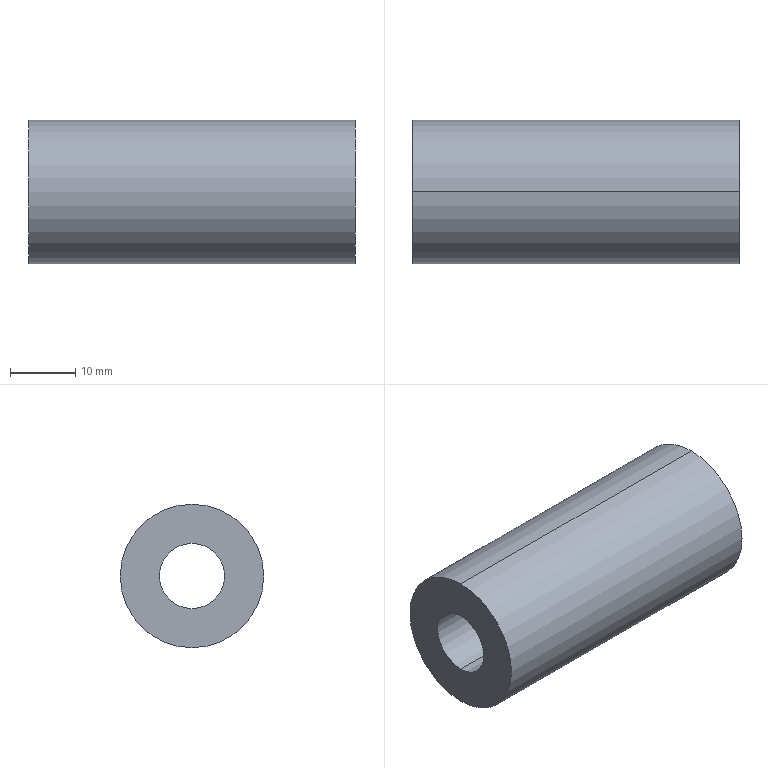Part | SolidWorks | features BaseBody 1 | 1 solid | 6 faces | box 50 x 22 x 22 mm | volume 15080 mm3 | cylinder 4 | plane 2 | commonest cylinder face diameters 10 x2 22 x2
STEP:
#1=CARTESIAN_POINT('',(-84.,58.,57.));
#2=VERTEX_POINT('',#1);
#3=CARTESIAN_POINT('',(-84.,58.,35.));
#4=VERTEX_POINT('',#3);
#5=CARTESIAN_POINT('',(-84.,58.,46.));
#6=DIRECTION('',(-1.,0.,0.));
#7=DIRECTION('',(0.,0.,1.));
#8=AXIS2_PLACEMENT_3D('',#5,#6,#7);
#9=CIRCLE('',#8,11.);
#10=EDGE_CURVE('',#2,#4,#9,.T.);
#11=ORIENTED_EDGE('',*,*,#10,.T.);
#12=CARTESIAN_POINT('',(-134.,58.,35.));
#13=VERTEX_POINT('',#12);
#14=CARTESIAN_POINT('',(-84.,58.,35.));
#15=DIRECTION('',(-1.,0.,0.));
#16=VECTOR('',#15,1000.);
#17=LINE('',#14,#16);
#18=EDGE_CURVE('',#4,#13,#17,.T.);
#19=ORIENTED_EDGE('',*,*,#18,.T.);
#20=CARTESIAN_POINT('',(-134.,58.,57.));
#21=VERTEX_POINT('',#20);
#22=CARTESIAN_POINT('',(-134.,58.,46.));
#23=DIRECTION('',(1.,0.,0.));
#24=DIRECTION('',(0.,0.,1.));
#25=AXIS2_PLACEMENT_3D('',#22,#23,#24);
#26=CIRCLE('',#25,11.);
#27=EDGE_CURVE('',#13,#21,#26,.T.);
#28=ORIENTED_EDGE('',*,*,#27,.T.);
#29=CARTESIAN_POINT('',(-84.,58.,57.));
#30=DIRECTION('',(-1.,0.,0.));
#31=VECTOR('',#30,1000.);
#32=LINE('',#29,#31);
#33=EDGE_CURVE('',#2,#21,#32,.T.);
#34=ORIENTED_EDGE('',*,*,#33,.F.);
#35=EDGE_LOOP('',(#11,#19,#28,#34));
#36=FACE_OUTER_BOUND('',#35,.T.);
#37=CARTESIAN_POINT('',(-84.,58.,46.));
#38=DIRECTION('',(-1.,0.,0.));
#39=DIRECTION('',(0.,0.,1.));
#40=AXIS2_PLACEMENT_3D('',#37,#38,#39);
#41=CYLINDRICAL_SURFACE('',#40,11.);
#42=ADVANCED_FACE('',(#36),#41,.T.);
#43=CARTESIAN_POINT('',(-84.,58.,41.));
#44=VERTEX_POINT('',#43);
#45=CARTESIAN_POINT('',(-84.,58.,51.));
#46=VERTEX_POINT('',#45);
#47=CARTESIAN_POINT('',(-84.,58.,46.));
#48=DIRECTION('',(-1.,0.,0.));
#49=DIRECTION('',(0.,0.,1.));
#50=AXIS2_PLACEMENT_3D('',#47,#48,#49);
#51=CIRCLE('',#50,5.);
#52=EDGE_CURVE('',#44,#46,#51,.T.);
#53=ORIENTED_EDGE('',*,*,#52,.F.);
#54=CARTESIAN_POINT('',(-134.,58.,41.));
#55=VERTEX_POINT('',#54);
#56=CARTESIAN_POINT('',(-84.,58.,41.));
#57=DIRECTION('',(-1.,0.,0.));
#58=VECTOR('',#57,1000.);
#59=LINE('',#56,#58);
#60=EDGE_CURVE('',#44,#55,#59,.T.);
#61=ORIENTED_EDGE('',*,*,#60,.T.);
#62=CARTESIAN_POINT('',(-134.,58.,51.));
#63=VERTEX_POINT('',#62);
#64=CARTESIAN_POINT('',(-134.,58.,46.));
#65=DIRECTION('',(-1.,0.,0.));
#66=DIRECTION('',(0.,0.,1.));
#67=AXIS2_PLACEMENT_3D('',#64,#65,#66);
#68=CIRCLE('',#67,5.);
#69=EDGE_CURVE('',#55,#63,#68,.T.);
#70=ORIENTED_EDGE('',*,*,#69,.T.);
#71=CARTESIAN_POINT('',(-84.,58.,51.));
#72=DIRECTION('',(-1.,0.,0.));
#73=VECTOR('',#72,1000.);
#74=LINE('',#71,#73);
#75=EDGE_CURVE('',#46,#63,#74,.T.);
#76=ORIENTED_EDGE('',*,*,#75,.F.);
#77=EDGE_LOOP('',(#53,#61,#70,#76));
#78=FACE_OUTER_BOUND('',#77,.T.);
#79=CARTESIAN_POINT('',(-84.,58.,46.));
#80=DIRECTION('',(-1.,0.,0.));
#81=DIRECTION('',(0.,0.,1.));
#82=AXIS2_PLACEMENT_3D('',#79,#80,#81);
#83=CYLINDRICAL_SURFACE('',#82,5.);
#84=ADVANCED_FACE('',(#78),#83,.F.);
#85=ORIENTED_EDGE('',*,*,#18,.F.);
#86=CARTESIAN_POINT('',(-84.,58.,46.));
#87=DIRECTION('',(-1.,0.,0.));
#88=DIRECTION('',(0.,0.,1.));
#89=AXIS2_PLACEMENT_3D('',#86,#87,#88);
#90=CIRCLE('',#89,11.);
#91=EDGE_CURVE('',#4,#2,#90,.T.);
#92=ORIENTED_EDGE('',*,*,#91,.T.);
#93=ORIENTED_EDGE('',*,*,#33,.T.);
#94=CARTESIAN_POINT('',(-134.,58.,46.));
#95=DIRECTION('',(1.,0.,0.));
#96=DIRECTION('',(0.,0.,1.));
#97=AXIS2_PLACEMENT_3D('',#94,#95,#96);
#98=CIRCLE('',#97,11.);
#99=EDGE_CURVE('',#21,#13,#98,.T.);
#100=ORIENTED_EDGE('',*,*,#99,.T.);
#101=EDGE_LOOP('',(#85,#92,#93,#100));
#102=FACE_OUTER_BOUND('',#101,.T.);
#103=CARTESIAN_POINT('',(-84.,58.,46.));
#104=DIRECTION('',(-1.,0.,0.));
#105=DIRECTION('',(0.,0.,1.));
#106=AXIS2_PLACEMENT_3D('',#103,#104,#105);
#107=CYLINDRICAL_SURFACE('',#106,11.);
#108=ADVANCED_FACE('',(#102),#107,.T.);
#109=CARTESIAN_POINT('',(-84.,58.,46.));
#110=DIRECTION('',(-1.,0.,0.));
#111=DIRECTION('',(0.,0.,1.));
#112=AXIS2_PLACEMENT_3D('',#109,#110,#111);
#113=CIRCLE('',#112,5.);
#114=EDGE_CURVE('',#46,#44,#113,.T.);
#115=ORIENTED_EDGE('',*,*,#114,.T.);
#116=ORIENTED_EDGE('',*,*,#52,.T.);
#117=EDGE_LOOP('',(#115,#116));
#118=FACE_BOUND('',#117,.T.);
#119=ORIENTED_EDGE('',*,*,#10,.F.);
#120=ORIENTED_EDGE('',*,*,#91,.F.);
#121=EDGE_LOOP('',(#119,#120));
#122=FACE_OUTER_BOUND('',#121,.T.);
#123=CARTESIAN_POINT('',(-84.,58.,46.));
#124=DIRECTION('',(1.,0.,0.));
#125=DIRECTION('',(0.,0.,-1.));
#126=AXIS2_PLACEMENT_3D('',#123,#124,#125);
#127=PLANE('',#126);
#128=ADVANCED_FACE('',(#118,#122),#127,.T.);
#129=CARTESIAN_POINT('',(-134.,58.,46.));
#130=DIRECTION('',(-1.,0.,0.));
#131=DIRECTION('',(0.,0.,1.));
#132=AXIS2_PLACEMENT_3D('',#129,#130,#131);
#133=CIRCLE('',#132,5.);
#134=EDGE_CURVE('',#63,#55,#133,.T.);
#135=ORIENTED_EDGE('',*,*,#134,.F.);
#136=ORIENTED_EDGE('',*,*,#69,.F.);
#137=EDGE_LOOP('',(#135,#136));
#138=FACE_BOUND('',#137,.T.);
#139=ORIENTED_EDGE('',*,*,#99,.F.);
#140=ORIENTED_EDGE('',*,*,#27,.F.);
#141=EDGE_LOOP('',(#139,#140));
#142=FACE_OUTER_BOUND('',#141,.T.);
#143=CARTESIAN_POINT('',(-134.,58.,46.));
#144=DIRECTION('',(1.,0.,0.));
#145=DIRECTION('',(0.,0.,-1.));
#146=AXIS2_PLACEMENT_3D('',#143,#144,#145);
#147=PLANE('',#146);
#148=ADVANCED_FACE('',(#138,#142),#147,.F.);
#149=ORIENTED_EDGE('',*,*,#60,.F.);
#150=ORIENTED_EDGE('',*,*,#114,.F.);
#151=ORIENTED_EDGE('',*,*,#75,.T.);
#152=ORIENTED_EDGE('',*,*,#134,.T.);
#153=EDGE_LOOP('',(#149,#150,#151,#152));
#154=FACE_OUTER_BOUND('',#153,.T.);
#155=CARTESIAN_POINT('',(-84.,58.,46.));
#156=DIRECTION('',(-1.,0.,0.));
#157=DIRECTION('',(0.,0.,1.));
#158=AXIS2_PLACEMENT_3D('',#155,#156,#157);
#159=CYLINDRICAL_SURFACE('',#158,5.);
#160=ADVANCED_FACE('',(#154),#159,.F.);
#161=CLOSED_SHELL('',(#42,#84,#108,#128,#148,#160));
#162=MANIFOLD_SOLID_BREP('',#161);
#163=CARTESIAN_POINT('',(0.,0.,0.));
#164=DIRECTION('',(0.,0.,1.));
#165=DIRECTION('',(1.,0.,0.));
#166=AXIS2_PLACEMENT_3D('',#163,#164,#165);
#167=(LENGTH_UNIT()NAMED_UNIT(*)SI_UNIT(.MILLI.,.METRE.));
#168=UNCERTAINTY_MEASURE_WITH_UNIT(LENGTH_MEASURE(0.00001),#167,'','');
#169=(NAMED_UNIT(*)PLANE_ANGLE_UNIT()SI_UNIT($,.RADIAN.));
#170=(NAMED_UNIT(*)SI_UNIT($,.STERADIAN.)SOLID_ANGLE_UNIT());
#171=(GEOMETRIC_REPRESENTATION_CONTEXT(3)GLOBAL_UNCERTAINTY_ASSIGNED_CONTEXT((#168))GLOBAL_UNIT_ASSIGNED_CONTEXT((#167,#169,#170))REPRESENTATION_CONTEXT('',''));
#172=ADVANCED_BREP_SHAPE_REPRESENTATION('',(#162,#166),#171);